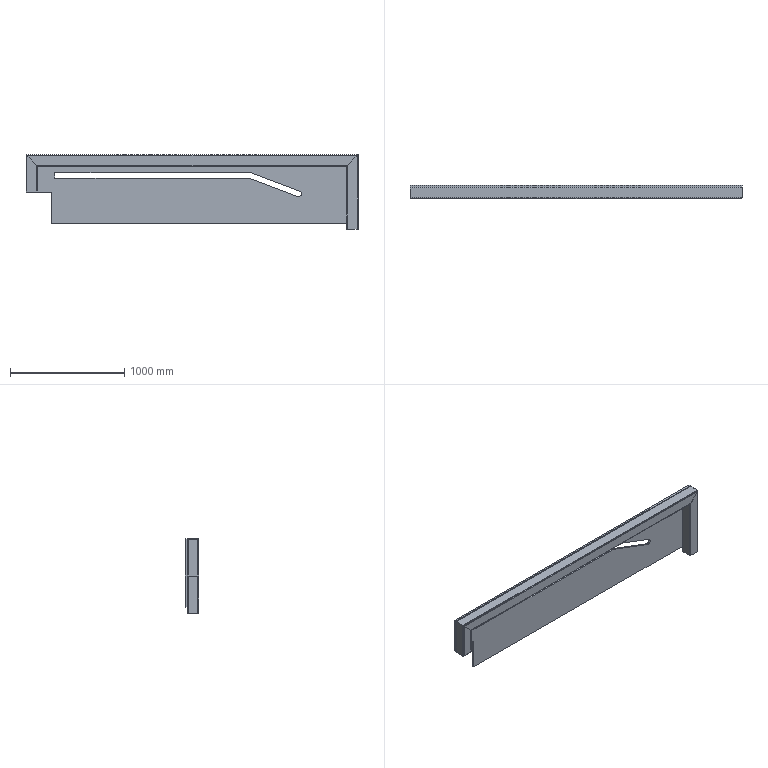Part | STEP file | Mirror rail_Default<Machined> | 4 solids | 70 faces | box 2900 x 115 x 650 mm | volume 29036229 mm3 | plane 43 | cylinder 27 | commonest cylinder face diameters 8 x12 16 x12 50 x3